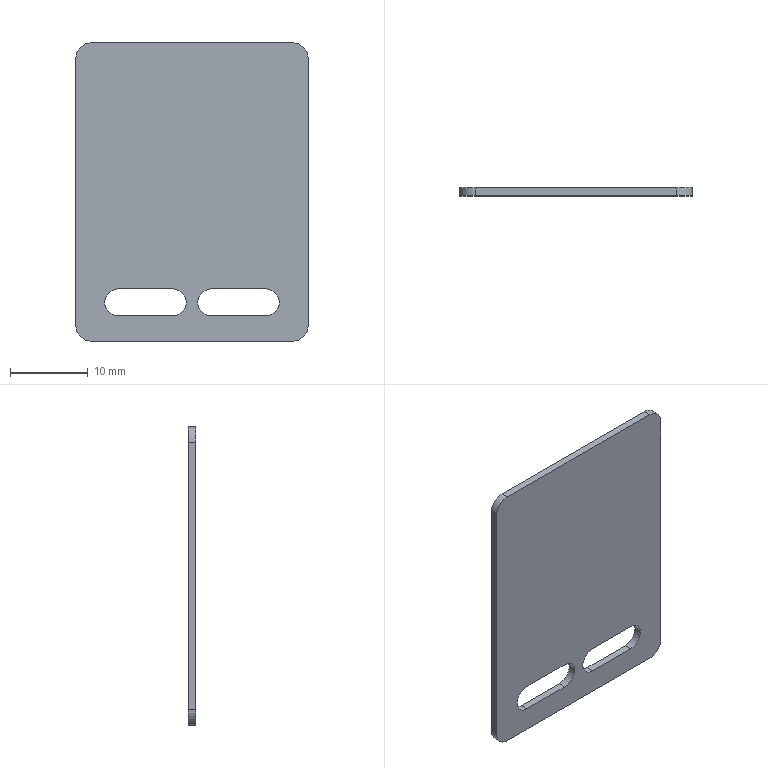Part | STEP file | 1 solid | 18 faces | box 30 x 1 x 38.5 mm | volume 1083 mm3 | plane 10 | cylinder 8 | commonest cylinder face diameters 3.5 x4 4 x4
STEP:
#1=CARTESIAN_POINT('',(0.,0.,0.));
#2=DIRECTION('',(0.,0.,1.));
#3=DIRECTION('',(1.,0.,0.));
#4=AXIS2_PLACEMENT_3D('',#1,#2,#3);
#5=CARTESIAN_POINT('',(-15.,-1.,2.));
#6=VERTEX_POINT('',#5);
#7=CARTESIAN_POINT('',(-13.,-1.,0.));
#8=VERTEX_POINT('',#7);
#9=CARTESIAN_POINT('',(-13.,-1.,2.));
#10=DIRECTION('',(0.,-1.,0.));
#11=DIRECTION('',(-1.,0.,0.));
#12=AXIS2_PLACEMENT_3D('',#9,#10,#11);
#13=CIRCLE('',#12,2.);
#14=CARTESIAN_POINT('',(-13.,0.,2.));
#15=DIRECTION('',(0.,1.,0.));
#16=DIRECTION('',(0.,0.,1.));
#17=AXIS2_PLACEMENT_3D('',#14,#15,#16);
#18=CYLINDRICAL_SURFACE('',#17,2.);
#19=CARTESIAN_POINT('',(4.712,-1.));
#20=DIRECTION('',(-1.,0.));
#21=VECTOR('',#20,1.);
#22=LINE('',#19,#21);
#23=(GEOMETRIC_REPRESENTATION_CONTEXT(2)PARAMETRIC_REPRESENTATION_CONTEXT()REPRESENTATION_CONTEXT('',''));
#24=DEFINITIONAL_REPRESENTATION('',(#22),#23);
#25=PCURVE('',#18,#24);
#26=CARTESIAN_POINT('',(-15.,-1.,38.5));
#27=DIRECTION('',(0.,1.,0.));
#28=DIRECTION('',(-1.,0.,0.));
#29=AXIS2_PLACEMENT_3D('',#26,#27,#28);
#30=PLANE('',#29);
#31=CARTESIAN_POINT('',(0.,-36.5));
#32=CARTESIAN_POINT('',(0.,-39.964));
#33=CARTESIAN_POINT('',(-3.,-38.232));
#34=CARTESIAN_POINT('',(-6.,-36.5));
#35=CARTESIAN_POINT('',(-3.,-34.768));
#36=CARTESIAN_POINT('',(0.,-33.036));
#37=CARTESIAN_POINT('',(0.,-36.5));
#38=(BOUNDED_CURVE()B_SPLINE_CURVE(2,(#31,#32,#33,#34,#35,#36,#37),.UNSPECIFIED.,.T.,.F.)B_SPLINE_CURVE_WITH_KNOTS((1,2,2,2,2,1),(-2.094,0.,2.094,4.189,6.283,8.378),.UNSPECIFIED.)CURVE()GEOMETRIC_REPRESENTATION_ITEM()RATIONAL_B_SPLINE_CURVE((1.,0.5,1.,0.5,1.,0.5,1.))REPRESENTATION_ITEM(''));
#39=(GEOMETRIC_REPRESENTATION_CONTEXT(2)PARAMETRIC_REPRESENTATION_CONTEXT()REPRESENTATION_CONTEXT('',''));
#40=DEFINITIONAL_REPRESENTATION('',(#38),#39);
#41=PCURVE('',#30,#40);
#42=SURFACE_CURVE('',#13,(#25,#41),.PCURVE_S1.);
#43=EDGE_CURVE('',#6,#8,#42,.T.);
#44=ORIENTED_EDGE('',*,*,#43,.F.);
#45=CARTESIAN_POINT('',(-15.,0.,2.));
#46=VERTEX_POINT('',#45);
#47=CARTESIAN_POINT('',(-15.,-1.,2.));
#48=DIRECTION('',(0.,-1.,0.));
#49=VECTOR('',#48,1.);
#50=LINE('',#47,#49);
#51=CARTESIAN_POINT('',(4.712,-1.));
#52=DIRECTION('',(0.,-1.));
#53=VECTOR('',#52,1.);
#54=LINE('',#51,#53);
#55=(GEOMETRIC_REPRESENTATION_CONTEXT(2)PARAMETRIC_REPRESENTATION_CONTEXT()REPRESENTATION_CONTEXT('',''));
#56=DEFINITIONAL_REPRESENTATION('',(#54),#55);
#57=PCURVE('',#18,#56);
#58=CARTESIAN_POINT('',(-15.,-1.,38.5));
#59=DIRECTION('',(-1.,0.,0.));
#60=DIRECTION('',(0.,0.,1.));
#61=AXIS2_PLACEMENT_3D('',#58,#59,#60);
#62=PLANE('',#61);
#63=CARTESIAN_POINT('',(-36.5,0.));
#64=DIRECTION('',(0.,-1.));
#65=VECTOR('',#64,1.);
#66=LINE('',#63,#65);
#67=(GEOMETRIC_REPRESENTATION_CONTEXT(2)PARAMETRIC_REPRESENTATION_CONTEXT()REPRESENTATION_CONTEXT('',''));
#68=DEFINITIONAL_REPRESENTATION('',(#66),#67);
#69=PCURVE('',#62,#68);
#70=SURFACE_CURVE('',#50,(#57,#69),.PCURVE_S1.);
#71=EDGE_CURVE('',#46,#6,#70,.T.);
#72=ORIENTED_EDGE('',*,*,#71,.F.);
#73=CARTESIAN_POINT('',(-13.,0.,0.));
#74=VERTEX_POINT('',#73);
#75=CARTESIAN_POINT('',(-13.,0.,2.));
#76=DIRECTION('',(0.,1.,0.));
#77=DIRECTION('',(-1.,0.,0.));
#78=AXIS2_PLACEMENT_3D('',#75,#76,#77);
#79=CIRCLE('',#78,2.);
#80=CARTESIAN_POINT('',(-1.571,0.));
#81=DIRECTION('',(1.,0.));
#82=VECTOR('',#81,1.);
#83=LINE('',#80,#82);
#84=(GEOMETRIC_REPRESENTATION_CONTEXT(2)PARAMETRIC_REPRESENTATION_CONTEXT()REPRESENTATION_CONTEXT('',''));
#85=DEFINITIONAL_REPRESENTATION('',(#83),#84);
#86=PCURVE('',#18,#85);
#87=CARTESIAN_POINT('',(-15.,0.,38.5));
#88=DIRECTION('',(0.,1.,0.));
#89=DIRECTION('',(-1.,0.,0.));
#90=AXIS2_PLACEMENT_3D('',#87,#88,#89);
#91=PLANE('',#90);
#92=CARTESIAN_POINT('',(-2.,-36.5));
#93=DIRECTION('',(1.,0.));
#94=AXIS2_PLACEMENT_2D('',#92,#93);
#95=CIRCLE('',#94,2.);
#96=(GEOMETRIC_REPRESENTATION_CONTEXT(2)PARAMETRIC_REPRESENTATION_CONTEXT()REPRESENTATION_CONTEXT('',''));
#97=DEFINITIONAL_REPRESENTATION('',(#95),#96);
#98=PCURVE('',#91,#97);
#99=SURFACE_CURVE('',#79,(#86,#98),.PCURVE_S1.);
#100=EDGE_CURVE('',#74,#46,#99,.T.);
#101=ORIENTED_EDGE('',*,*,#100,.F.);
#102=CARTESIAN_POINT('',(-13.,0.,0.));
#103=DIRECTION('',(0.,1.,0.));
#104=VECTOR('',#103,1.);
#105=LINE('',#102,#104);
#106=CARTESIAN_POINT('',(3.142,0.));
#107=DIRECTION('',(0.,1.));
#108=VECTOR('',#107,1.);
#109=LINE('',#106,#108);
#110=(GEOMETRIC_REPRESENTATION_CONTEXT(2)PARAMETRIC_REPRESENTATION_CONTEXT()REPRESENTATION_CONTEXT('',''));
#111=DEFINITIONAL_REPRESENTATION('',(#109),#110);
#112=PCURVE('',#18,#111);
#113=CARTESIAN_POINT('',(0.,0.,0.));
#114=DIRECTION('',(0.,0.,-1.));
#115=DIRECTION('',(-1.,0.,0.));
#116=AXIS2_PLACEMENT_3D('',#113,#114,#115);
#117=PLANE('',#116);
#118=CARTESIAN_POINT('',(13.,0.));
#119=DIRECTION('',(0.,1.));
#120=VECTOR('',#119,1.);
#121=LINE('',#118,#120);
#122=(GEOMETRIC_REPRESENTATION_CONTEXT(2)PARAMETRIC_REPRESENTATION_CONTEXT()REPRESENTATION_CONTEXT('',''));
#123=DEFINITIONAL_REPRESENTATION('',(#121),#122);
#124=PCURVE('',#117,#123);
#125=SURFACE_CURVE('',#105,(#112,#124),.PCURVE_S1.);
#126=EDGE_CURVE('',#8,#74,#125,.T.);
#127=ORIENTED_EDGE('',*,*,#126,.F.);
#128=EDGE_LOOP('',(#44,#72,#101,#127));
#129=FACE_BOUND('',#128,.T.);
#130=ADVANCED_FACE('',(#129),#18,.T.);
#131=CARTESIAN_POINT('',(15.,0.,2.));
#132=VERTEX_POINT('',#131);
#133=CARTESIAN_POINT('',(13.,0.,0.));
#134=VERTEX_POINT('',#133);
#135=CARTESIAN_POINT('',(13.,0.,2.));
#136=DIRECTION('',(0.,1.,0.));
#137=DIRECTION('',(-1.,0.,0.));
#138=AXIS2_PLACEMENT_3D('',#135,#136,#137);
#139=CIRCLE('',#138,2.);
#140=CARTESIAN_POINT('',(13.,0.,2.));
#141=DIRECTION('',(0.,-1.,0.));
#142=DIRECTION('',(0.,0.,-1.));
#143=AXIS2_PLACEMENT_3D('',#140,#141,#142);
#144=CYLINDRICAL_SURFACE('',#143,2.);
#145=CARTESIAN_POINT('',(4.712,0.));
#146=DIRECTION('',(-1.,0.));
#147=VECTOR('',#146,1.);
#148=LINE('',#145,#147);
#149=(GEOMETRIC_REPRESENTATION_CONTEXT(2)PARAMETRIC_REPRESENTATION_CONTEXT()REPRESENTATION_CONTEXT('',''));
#150=DEFINITIONAL_REPRESENTATION('',(#148),#149);
#151=PCURVE('',#144,#150);
#152=CARTESIAN_POINT('',(-28.,-36.5));
#153=DIRECTION('',(1.,0.));
#154=AXIS2_PLACEMENT_2D('',#152,#153);
#155=CIRCLE('',#154,2.);
#156=(GEOMETRIC_REPRESENTATION_CONTEXT(2)PARAMETRIC_REPRESENTATION_CONTEXT()REPRESENTATION_CONTEXT('',''));
#157=DEFINITIONAL_REPRESENTATION('',(#155),#156);
#158=PCURVE('',#91,#157);
#159=SURFACE_CURVE('',#139,(#151,#158),.PCURVE_S1.);
#160=EDGE_CURVE('',#132,#134,#159,.T.);
#161=ORIENTED_EDGE('',*,*,#160,.F.);
#162=CARTESIAN_POINT('',(15.,-1.,2.));
#163=VERTEX_POINT('',#162);
#164=CARTESIAN_POINT('',(15.,0.,2.));
#165=DIRECTION('',(0.,1.,0.));
#166=VECTOR('',#165,1.);
#167=LINE('',#164,#166);
#168=CARTESIAN_POINT('',(1.571,0.));
#169=DIRECTION('',(0.,-1.));
#170=VECTOR('',#169,1.);
#171=LINE('',#168,#170);
#172=(GEOMETRIC_REPRESENTATION_CONTEXT(2)PARAMETRIC_REPRESENTATION_CONTEXT()REPRESENTATION_CONTEXT('',''));
#173=DEFINITIONAL_REPRESENTATION('',(#171),#172);
#174=PCURVE('',#144,#173);
#175=CARTESIAN_POINT('',(15.,0.,38.5));
#176=DIRECTION('',(1.,0.,0.));
#177=DIRECTION('',(0.,0.,-1.));
#178=AXIS2_PLACEMENT_3D('',#175,#176,#177);
#179=PLANE('',#178);
#180=CARTESIAN_POINT('',(36.5,0.));
#181=DIRECTION('',(0.,1.));
#182=VECTOR('',#181,1.);
#183=LINE('',#180,#182);
#184=(GEOMETRIC_REPRESENTATION_CONTEXT(2)PARAMETRIC_REPRESENTATION_CONTEXT()REPRESENTATION_CONTEXT('',''));
#185=DEFINITIONAL_REPRESENTATION('',(#183),#184);
#186=PCURVE('',#179,#185);
#187=SURFACE_CURVE('',#167,(#174,#186),.PCURVE_S1.);
#188=EDGE_CURVE('',#163,#132,#187,.T.);
#189=ORIENTED_EDGE('',*,*,#188,.F.);
#190=CARTESIAN_POINT('',(13.,-1.,0.));
#191=VERTEX_POINT('',#190);
#192=CARTESIAN_POINT('',(13.,-1.,2.));
#193=DIRECTION('',(0.,-1.,0.));
#194=DIRECTION('',(-1.,0.,0.));
#195=AXIS2_PLACEMENT_3D('',#192,#193,#194);
#196=CIRCLE('',#195,2.);
#197=CARTESIAN_POINT('',(-1.571,1.));
#198=DIRECTION('',(1.,0.));
#199=VECTOR('',#198,1.);
#200=LINE('',#197,#199);
#201=(GEOMETRIC_REPRESENTATION_CONTEXT(2)PARAMETRIC_REPRESENTATION_CONTEXT()REPRESENTATION_CONTEXT('',''));
#202=DEFINITIONAL_REPRESENTATION('',(#200),#201);
#203=PCURVE('',#144,#202);
#204=CARTESIAN_POINT('',(-26.,-36.5));
#205=CARTESIAN_POINT('',(-26.,-39.964));
#206=CARTESIAN_POINT('',(-29.,-38.232));
#207=CARTESIAN_POINT('',(-32.,-36.5));
#208=CARTESIAN_POINT('',(-29.,-34.768));
#209=CARTESIAN_POINT('',(-26.,-33.036));
#210=CARTESIAN_POINT('',(-26.,-36.5));
#211=(BOUNDED_CURVE()B_SPLINE_CURVE(2,(#204,#205,#206,#207,#208,#209,#210),.UNSPECIFIED.,.T.,.F.)B_SPLINE_CURVE_WITH_KNOTS((1,2,2,2,2,1),(-2.094,0.,2.094,4.189,6.283,8.378),.UNSPECIFIED.)CURVE()GEOMETRIC_REPRESENTATION_ITEM()RATIONAL_B_SPLINE_CURVE((1.,0.5,1.,0.5,1.,0.5,1.))REPRESENTATION_ITEM(''));
#212=(GEOMETRIC_REPRESENTATION_CONTEXT(2)PARAMETRIC_REPRESENTATION_CONTEXT()REPRESENTATION_CONTEXT('',''));
#213=DEFINITIONAL_REPRESENTATION('',(#211),#212);
#214=PCURVE('',#30,#213);
#215=SURFACE_CURVE('',#196,(#203,#214),.PCURVE_S1.);
#216=EDGE_CURVE('',#191,#163,#215,.T.);
#217=ORIENTED_EDGE('',*,*,#216,.F.);
#218=CARTESIAN_POINT('',(13.,0.,0.));
#219=DIRECTION('',(0.,-1.,0.));
#220=VECTOR('',#219,1.);
#221=LINE('',#218,#220);
#222=CARTESIAN_POINT('',(0.,0.));
#223=DIRECTION('',(0.,1.));
#224=VECTOR('',#223,1.);
#225=LINE('',#222,#224);
#226=(GEOMETRIC_REPRESENTATION_CONTEXT(2)PARAMETRIC_REPRESENTATION_CONTEXT()REPRESENTATION_CONTEXT('',''));
#227=DEFINITIONAL_REPRESENTATION('',(#225),#226);
#228=PCURVE('',#144,#227);
#229=CARTESIAN_POINT('',(-13.,0.));
#230=DIRECTION('',(0.,-1.));
#231=VECTOR('',#230,1.);
#232=LINE('',#229,#231);
#233=(GEOMETRIC_REPRESENTATION_CONTEXT(2)PARAMETRIC_REPRESENTATION_CONTEXT()REPRESENTATION_CONTEXT('',''));
#234=DEFINITIONAL_REPRESENTATION('',(#232),#233);
#235=PCURVE('',#117,#234);
#236=SURFACE_CURVE('',#221,(#228,#235),.PCURVE_S1.);
#237=EDGE_CURVE('',#134,#191,#236,.T.);
#238=ORIENTED_EDGE('',*,*,#237,.F.);
#239=EDGE_LOOP('',(#161,#189,#217,#238));
#240=FACE_BOUND('',#239,.T.);
#241=ADVANCED_FACE('',(#240),#144,.T.);
#242=CARTESIAN_POINT('',(-13.,-1.,38.5));
#243=VERTEX_POINT('',#242);
#244=CARTESIAN_POINT('',(-15.,-1.,36.5));
#245=VERTEX_POINT('',#244);
#246=CARTESIAN_POINT('',(-13.,-1.,36.5));
#247=DIRECTION('',(0.,-1.,0.));
#248=DIRECTION('',(-1.,0.,0.));
#249=AXIS2_PLACEMENT_3D('',#246,#247,#248);
#250=CIRCLE('',#249,2.);
#251=CARTESIAN_POINT('',(-13.,-1.,36.5));
#252=DIRECTION('',(0.,-1.,0.));
#253=DIRECTION('',(0.,0.,-1.));
#254=AXIS2_PLACEMENT_3D('',#251,#252,#253);
#255=CYLINDRICAL_SURFACE('',#254,2.);
#256=CARTESIAN_POINT('',(-1.571,0.));
#257=DIRECTION('',(1.,0.));
#258=VECTOR('',#257,1.);
#259=LINE('',#256,#258);
#260=(GEOMETRIC_REPRESENTATION_CONTEXT(2)PARAMETRIC_REPRESENTATION_CONTEXT()REPRESENTATION_CONTEXT('',''));
#261=DEFINITIONAL_REPRESENTATION('',(#259),#260);
#262=PCURVE('',#255,#261);
#263=CARTESIAN_POINT('',(0.,-2.));
#264=CARTESIAN_POINT('',(0.,-5.464));
#265=CARTESIAN_POINT('',(-3.,-3.732));
#266=CARTESIAN_POINT('',(-6.,-2.));
#267=CARTESIAN_POINT('',(-3.,-0.2679));
#268=CARTESIAN_POINT('',(0.,1.464));
#269=CARTESIAN_POINT('',(0.,-2.));
#270=(BOUNDED_CURVE()B_SPLINE_CURVE(2,(#263,#264,#265,#266,#267,#268,#269),.UNSPECIFIED.,.T.,.F.)B_SPLINE_CURVE_WITH_KNOTS((1,2,2,2,2,1),(-2.094,0.,2.094,4.189,6.283,8.378),.UNSPECIFIED.)CURVE()GEOMETRIC_REPRESENTATION_ITEM()RATIONAL_B_SPLINE_CURVE((1.,0.5,1.,0.5,1.,0.5,1.))REPRESENTATION_ITEM(''));
#271=(GEOMETRIC_REPRESENTATION_CONTEXT(2)PARAMETRIC_REPRESENTATION_CONTEXT()REPRESENTATION_CONTEXT('',''));
#272=DEFINITIONAL_REPRESENTATION('',(#270),#271);
#273=PCURVE('',#30,#272);
#274=SURFACE_CURVE('',#250,(#262,#273),.PCURVE_S1.);
#275=EDGE_CURVE('',#243,#245,#274,.T.);
#276=ORIENTED_EDGE('',*,*,#275,.F.);
#277=CARTESIAN_POINT('',(-13.,0.,38.5));
#278=VERTEX_POINT('',#277);
#279=CARTESIAN_POINT('',(-13.,-1.,38.5));
#280=DIRECTION('',(0.,-1.,0.));
#281=VECTOR('',#280,1.);
#282=LINE('',#279,#281);
#283=CARTESIAN_POINT('',(3.142,0.));
#284=DIRECTION('',(0.,1.));
#285=VECTOR('',#284,1.);
#286=LINE('',#283,#285);
#287=(GEOMETRIC_REPRESENTATION_CONTEXT(2)PARAMETRIC_REPRESENTATION_CONTEXT()REPRESENTATION_CONTEXT('',''));
#288=DEFINITIONAL_REPRESENTATION('',(#286),#287);
#289=PCURVE('',#255,#288);
#290=CARTESIAN_POINT('',(0.,0.,38.5));
#291=DIRECTION('',(0.,0.,-1.));
#292=DIRECTION('',(-1.,0.,0.));
#293=AXIS2_PLACEMENT_3D('',#290,#291,#292);
#294=PLANE('',#293);
#295=CARTESIAN_POINT('',(13.,-1.));
#296=DIRECTION('',(0.,-1.));
#297=VECTOR('',#296,1.);
#298=LINE('',#295,#297);
#299=(GEOMETRIC_REPRESENTATION_CONTEXT(2)PARAMETRIC_REPRESENTATION_CONTEXT()REPRESENTATION_CONTEXT('',''));
#300=DEFINITIONAL_REPRESENTATION('',(#298),#299);
#301=PCURVE('',#294,#300);
#302=SURFACE_CURVE('',#282,(#289,#301),.PCURVE_S1.);
#303=EDGE_CURVE('',#278,#243,#302,.T.);
#304=ORIENTED_EDGE('',*,*,#303,.F.);
#305=CARTESIAN_POINT('',(-15.,0.,36.5));
#306=VERTEX_POINT('',#305);
#307=CARTESIAN_POINT('',(-13.,0.,36.5));
#308=DIRECTION('',(0.,1.,0.));
#309=DIRECTION('',(-1.,0.,0.));
#310=AXIS2_PLACEMENT_3D('',#307,#308,#309);
#311=CIRCLE('',#310,2.);
#312=CARTESIAN_POINT('',(4.712,-1.));
#313=DIRECTION('',(-1.,0.));
#314=VECTOR('',#313,1.);
#315=LINE('',#312,#314);
#316=(GEOMETRIC_REPRESENTATION_CONTEXT(2)PARAMETRIC_REPRESENTATION_CONTEXT()REPRESENTATION_CONTEXT('',''));
#317=DEFINITIONAL_REPRESENTATION('',(#315),#316);
#318=PCURVE('',#255,#317);
#319=CARTESIAN_POINT('',(-2.,-2.));
#320=DIRECTION('',(1.,0.));
#321=AXIS2_PLACEMENT_2D('',#319,#320);
#322=CIRCLE('',#321,2.);
#323=(GEOMETRIC_REPRESENTATION_CONTEXT(2)PARAMETRIC_REPRESENTATION_CONTEXT()REPRESENTATION_CONTEXT('',''));
#324=DEFINITIONAL_REPRESENTATION('',(#322),#323);
#325=PCURVE('',#91,#324);
#326=SURFACE_CURVE('',#311,(#318,#325),.PCURVE_S1.);
#327=EDGE_CURVE('',#306,#278,#326,.T.);
#328=ORIENTED_EDGE('',*,*,#327,.F.);
#329=CARTESIAN_POINT('',(-15.,0.,36.5));
#330=DIRECTION('',(0.,1.,0.));
#331=VECTOR('',#330,1.);
#332=LINE('',#329,#331);
#333=CARTESIAN_POINT('',(4.712,-1.));
#334=DIRECTION('',(0.,-1.));
#335=VECTOR('',#334,1.);
#336=LINE('',#333,#335);
#337=(GEOMETRIC_REPRESENTATION_CONTEXT(2)PARAMETRIC_REPRESENTATION_CONTEXT()REPRESENTATION_CONTEXT('',''));
#338=DEFINITIONAL_REPRESENTATION('',(#336),#337);
#339=PCURVE('',#255,#338);
#340=CARTESIAN_POINT('',(-2.,1.));
#341=DIRECTION('',(0.,1.));
#342=VECTOR('',#341,1.);
#343=LINE('',#340,#342);
#344=(GEOMETRIC_REPRESENTATION_CONTEXT(2)PARAMETRIC_REPRESENTATION_CONTEXT()REPRESENTATION_CONTEXT('',''));
#345=DEFINITIONAL_REPRESENTATION('',(#343),#344);
#346=PCURVE('',#62,#345);
#347=SURFACE_CURVE('',#332,(#339,#346),.PCURVE_S1.);
#348=EDGE_CURVE('',#245,#306,#347,.T.);
#349=ORIENTED_EDGE('',*,*,#348,.F.);
#350=EDGE_LOOP('',(#276,#304,#328,#349));
#351=FACE_BOUND('',#350,.T.);
#352=ADVANCED_FACE('',(#351),#255,.T.);
#353=CARTESIAN_POINT('',(13.,0.,38.5));
#354=VERTEX_POINT('',#353);
#355=CARTESIAN_POINT('',(15.,0.,36.5));
#356=VERTEX_POINT('',#355);
#357=CARTESIAN_POINT('',(13.,0.,36.5));
#358=DIRECTION('',(0.,1.,0.));
#359=DIRECTION('',(-1.,0.,0.));
#360=AXIS2_PLACEMENT_3D('',#357,#358,#359);
#361=CIRCLE('',#360,2.);
#362=CARTESIAN_POINT('',(13.,0.,36.5));
#363=DIRECTION('',(0.,1.,0.));
#364=DIRECTION('',(0.,0.,1.));
#365=AXIS2_PLACEMENT_3D('',#362,#363,#364);
#366=CYLINDRICAL_SURFACE('',#365,2.);
#367=CARTESIAN_POINT('',(-1.571,0.));
#368=DIRECTION('',(1.,0.));
#369=VECTOR('',#368,1.);
#370=LINE('',#367,#369);
#371=(GEOMETRIC_REPRESENTATION_CONTEXT(2)PARAMETRIC_REPRESENTATION_CONTEXT()REPRESENTATION_CONTEXT('',''));
#372=DEFINITIONAL_REPRESENTATION('',(#370),#371);
#373=PCURVE('',#366,#372);
#374=CARTESIAN_POINT('',(-28.,-2.));
#375=DIRECTION('',(1.,0.));
#376=AXIS2_PLACEMENT_2D('',#374,#375);
#377=CIRCLE('',#376,2.);
#378=(GEOMETRIC_REPRESENTATION_CONTEXT(2)PARAMETRIC_REPRESENTATION_CONTEXT()REPRESENTATION_CONTEXT('',''));
#379=DEFINITIONAL_REPRESENTATION('',(#377),#378);
#380=PCURVE('',#91,#379);
#381=SURFACE_CURVE('',#361,(#373,#380),.PCURVE_S1.);
#382=EDGE_CURVE('',#354,#356,#381,.T.);
#383=ORIENTED_EDGE('',*,*,#382,.F.);
#384=CARTESIAN_POINT('',(13.,-1.,38.5));
#385=VERTEX_POINT('',#384);
#386=CARTESIAN_POINT('',(13.,0.,38.5));
#387=DIRECTION('',(0.,1.,0.));
#388=VECTOR('',#387,1.);
#389=LINE('',#386,#388);
#390=CARTESIAN_POINT('',(0.,0.));
#391=DIRECTION('',(0.,1.));
#392=VECTOR('',#391,1.);
#393=LINE('',#390,#392);
#394=(GEOMETRIC_REPRESENTATION_CONTEXT(2)PARAMETRIC_REPRESENTATION_CONTEXT()REPRESENTATION_CONTEXT('',''));
#395=DEFINITIONAL_REPRESENTATION('',(#393),#394);
#396=PCURVE('',#366,#395);
#397=CARTESIAN_POINT('',(-13.,0.));
#398=DIRECTION('',(0.,1.));
#399=VECTOR('',#398,1.);
#400=LINE('',#397,#399);
#401=(GEOMETRIC_REPRESENTATION_CONTEXT(2)PARAMETRIC_REPRESENTATION_CONTEXT()REPRESENTATION_CONTEXT('',''));
#402=DEFINITIONAL_REPRESENTATION('',(#400),#401);
#403=PCURVE('',#294,#402);
#404=SURFACE_CURVE('',#389,(#396,#403),.PCURVE_S1.);
#405=EDGE_CURVE('',#385,#354,#404,.T.);
#406=ORIENTED_EDGE('',*,*,#405,.F.);
#407=CARTESIAN_POINT('',(15.,-1.,36.5));
#408=VERTEX_POINT('',#407);
#409=CARTESIAN_POINT('',(13.,-1.,36.5));
#410=DIRECTION('',(0.,-1.,0.));
#411=DIRECTION('',(-1.,0.,0.));
#412=AXIS2_PLACEMENT_3D('',#409,#410,#411);
#413=CIRCLE('',#412,2.);
#414=CARTESIAN_POINT('',(4.712,-1.));
#415=DIRECTION('',(-1.,0.));
#416=VECTOR('',#415,1.);
#417=LINE('',#414,#416);
#418=(GEOMETRIC_REPRESENTATION_CONTEXT(2)PARAMETRIC_REPRESENTATION_CONTEXT()REPRESENTATION_CONTEXT('',''));
#419=DEFINITIONAL_REPRESENTATION('',(#417),#418);
#420=PCURVE('',#366,#419);
#421=CARTESIAN_POINT('',(-26.,-2.));
#422=CARTESIAN_POINT('',(-26.,-5.464));
#423=CARTESIAN_POINT('',(-29.,-3.732));
#424=CARTESIAN_POINT('',(-32.,-2.));
#425=CARTESIAN_POINT('',(-29.,-0.2679));
#426=CARTESIAN_POINT('',(-26.,1.464));
#427=CARTESIAN_POINT('',(-26.,-2.));
#428=(BOUNDED_CURVE()B_SPLINE_CURVE(2,(#421,#422,#423,#424,#425,#426,#427),.UNSPECIFIED.,.T.,.F.)B_SPLINE_CURVE_WITH_KNOTS((1,2,2,2,2,1),(-2.094,0.,2.094,4.189,6.283,8.378),.UNSPECIFIED.)CURVE()GEOMETRIC_REPRESENTATION_ITEM()RATIONAL_B_SPLINE_CURVE((1.,0.5,1.,0.5,1.,0.5,1.))REPRESENTATION_ITEM(''));
#429=(GEOMETRIC_REPRESENTATION_CONTEXT(2)PARAMETRIC_REPRESENTATION_CONTEXT()REPRESENTATION_CONTEXT('',''));
#430=DEFINITIONAL_REPRESENTATION('',(#428),#429);
#431=PCURVE('',#30,#430);
#432=SURFACE_CURVE('',#413,(#420,#431),.PCURVE_S1.);
#433=EDGE_CURVE('',#408,#385,#432,.T.);
#434=ORIENTED_EDGE('',*,*,#433,.F.);
#435=CARTESIAN_POINT('',(15.,-1.,36.5));
#436=DIRECTION('',(0.,-1.,0.));
#437=VECTOR('',#436,1.);
#438=LINE('',#435,#437);
#439=CARTESIAN_POINT('',(1.571,-1.));
#440=DIRECTION('',(0.,-1.));
#441=VECTOR('',#440,1.);
#442=LINE('',#439,#441);
#443=(GEOMETRIC_REPRESENTATION_CONTEXT(2)PARAMETRIC_REPRESENTATION_CONTEXT()REPRESENTATION_CONTEXT('',''));
#444=DEFINITIONAL_REPRESENTATION('',(#442),#443);
#445=PCURVE('',#366,#444);
#446=CARTESIAN_POINT('',(2.,-1.));
#447=DIRECTION('',(0.,-1.));
#448=VECTOR('',#447,1.);
#449=LINE('',#446,#448);
#450=(GEOMETRIC_REPRESENTATION_CONTEXT(2)PARAMETRIC_REPRESENTATION_CONTEXT()REPRESENTATION_CONTEXT('',''));
#451=DEFINITIONAL_REPRESENTATION('',(#449),#450);
#452=PCURVE('',#179,#451);
#453=SURFACE_CURVE('',#438,(#445,#452),.PCURVE_S1.);
#454=EDGE_CURVE('',#356,#408,#453,.T.);
#455=ORIENTED_EDGE('',*,*,#454,.F.);
#456=EDGE_LOOP('',(#383,#406,#434,#455));
#457=FACE_BOUND('',#456,.T.);
#458=ADVANCED_FACE('',(#457),#366,.T.);
#459=CARTESIAN_POINT('',(2.5,-1.,6.75));
#460=VERTEX_POINT('',#459);
#461=CARTESIAN_POINT('',(2.5,0.,6.75));
#462=VERTEX_POINT('',#461);
#463=CARTESIAN_POINT('',(2.5,-10.,6.75));
#464=DIRECTION('',(0.,1.,0.));
#465=VECTOR('',#464,1.);
#466=LINE('',#463,#465);
#467=CARTESIAN_POINT('',(2.5,-10.,6.75));
#468=DIRECTION('',(0.,0.,1.));
#469=DIRECTION('',(1.,0.,0.));
#470=AXIS2_PLACEMENT_3D('',#467,#468,#469);
#471=PLANE('',#470);
#472=CARTESIAN_POINT('',(0.,0.));
#473=DIRECTION('',(0.,1.));
#474=VECTOR('',#473,1.);
#475=LINE('',#472,#474);
#476=(GEOMETRIC_REPRESENTATION_CONTEXT(2)PARAMETRIC_REPRESENTATION_CONTEXT()REPRESENTATION_CONTEXT('',''));
#477=DEFINITIONAL_REPRESENTATION('',(#475),#476);
#478=PCURVE('',#471,#477);
#479=CARTESIAN_POINT('',(2.5,-10.,5.));
#480=DIRECTION('',(0.,1.,0.));
#481=DIRECTION('',(0.,0.,1.));
#482=AXIS2_PLACEMENT_3D('',#479,#480,#481);
#483=CYLINDRICAL_SURFACE('',#482,1.75);
#484=CARTESIAN_POINT('',(6.283,0.));
#485=DIRECTION('',(0.,1.));
#486=VECTOR('',#485,1.);
#487=LINE('',#484,#486);
#488=(GEOMETRIC_REPRESENTATION_CONTEXT(2)PARAMETRIC_REPRESENTATION_CONTEXT()REPRESENTATION_CONTEXT('',''));
#489=DEFINITIONAL_REPRESENTATION('',(#487),#488);
#490=PCURVE('',#483,#489);
#491=SURFACE_CURVE('',#466,(#478,#490),.PCURVE_S1.);
#492=EDGE_CURVE('',#460,#462,#491,.T.);
#493=ORIENTED_EDGE('',*,*,#492,.T.);
#494=CARTESIAN_POINT('',(9.5,0.,6.75));
#495=VERTEX_POINT('',#494);
#496=CARTESIAN_POINT('',(2.5,0.,6.75));
#497=DIRECTION('',(1.,0.,0.));
#498=VECTOR('',#497,1.);
#499=LINE('',#496,#498);
#500=CARTESIAN_POINT('',(0.,10.));
#501=DIRECTION('',(1.,0.));
#502=VECTOR('',#501,1.);
#503=LINE('',#500,#502);
#504=(GEOMETRIC_REPRESENTATION_CONTEXT(2)PARAMETRIC_REPRESENTATION_CONTEXT()REPRESENTATION_CONTEXT('',''));
#505=DEFINITIONAL_REPRESENTATION('',(#503),#504);
#506=PCURVE('',#471,#505);
#507=CARTESIAN_POINT('',(-17.5,-31.75));
#508=DIRECTION('',(-1.,0.));
#509=VECTOR('',#508,1.);
#510=LINE('',#507,#509);
#511=(GEOMETRIC_REPRESENTATION_CONTEXT(2)PARAMETRIC_REPRESENTATION_CONTEXT()REPRESENTATION_CONTEXT('',''));
#512=DEFINITIONAL_REPRESENTATION('',(#510),#511);
#513=PCURVE('',#91,#512);
#514=SURFACE_CURVE('',#499,(#506,#513),.PCURVE_S1.);
#515=EDGE_CURVE('',#462,#495,#514,.T.);
#516=ORIENTED_EDGE('',*,*,#515,.T.);
#517=CARTESIAN_POINT('',(9.5,-1.,6.75));
#518=VERTEX_POINT('',#517);
#519=CARTESIAN_POINT('',(9.5,-10.,6.75));
#520=DIRECTION('',(0.,1.,0.));
#521=VECTOR('',#520,1.);
#522=LINE('',#519,#521);
#523=CARTESIAN_POINT('',(7.,0.));
#524=DIRECTION('',(0.,1.));
#525=VECTOR('',#524,1.);
#526=LINE('',#523,#525);
#527=(GEOMETRIC_REPRESENTATION_CONTEXT(2)PARAMETRIC_REPRESENTATION_CONTEXT()REPRESENTATION_CONTEXT('',''));
#528=DEFINITIONAL_REPRESENTATION('',(#526),#527);
#529=PCURVE('',#471,#528);
#530=CARTESIAN_POINT('',(9.5,-10.,5.));
#531=DIRECTION('',(0.,1.,0.));
#532=DIRECTION('',(0.,0.,1.));
#533=AXIS2_PLACEMENT_3D('',#530,#531,#532);
#534=CYLINDRICAL_SURFACE('',#533,1.75);
#535=CARTESIAN_POINT('',(0.,0.));
#536=DIRECTION('',(0.,1.));
#537=VECTOR('',#536,1.);
#538=LINE('',#535,#537);
#539=(GEOMETRIC_REPRESENTATION_CONTEXT(2)PARAMETRIC_REPRESENTATION_CONTEXT()REPRESENTATION_CONTEXT('',''));
#540=DEFINITIONAL_REPRESENTATION('',(#538),#539);
#541=PCURVE('',#534,#540);
#542=SURFACE_CURVE('',#522,(#529,#541),.PCURVE_S1.);
#543=EDGE_CURVE('',#518,#495,#542,.T.);
#544=ORIENTED_EDGE('',*,*,#543,.F.);
#545=CARTESIAN_POINT('',(-15.,-1.,6.75));
#546=DIRECTION('',(1.,0.,0.));
#547=VECTOR('',#546,1.);
#548=LINE('',#545,#547);
#549=CARTESIAN_POINT('',(-17.5,9.));
#550=DIRECTION('',(1.,0.));
#551=VECTOR('',#550,1.);
#552=LINE('',#549,#551);
#553=(GEOMETRIC_REPRESENTATION_CONTEXT(2)PARAMETRIC_REPRESENTATION_CONTEXT()REPRESENTATION_CONTEXT('',''));
#554=DEFINITIONAL_REPRESENTATION('',(#552),#553);
#555=PCURVE('',#471,#554);
#556=CARTESIAN_POINT('',(0.,-31.75));
#557=DIRECTION('',(-1.,0.));
#558=VECTOR('',#557,1.);
#559=LINE('',#556,#558);
#560=(GEOMETRIC_REPRESENTATION_CONTEXT(2)PARAMETRIC_REPRESENTATION_CONTEXT()REPRESENTATION_CONTEXT('',''));
#561=DEFINITIONAL_REPRESENTATION('',(#559),#560);
#562=PCURVE('',#30,#561);
#563=SURFACE_CURVE('',#548,(#555,#562),.PCURVE_S1.);
#564=EDGE_CURVE('',#460,#518,#563,.T.);
#565=ORIENTED_EDGE('',*,*,#564,.F.);
#566=EDGE_LOOP('',(#493,#516,#544,#565));
#567=FACE_BOUND('',#566,.T.);
#568=ADVANCED_FACE('',(#567),#471,.F.);
#569=CARTESIAN_POINT('',(9.5,-1.,3.25));
#570=VERTEX_POINT('',#569);
#571=CARTESIAN_POINT('',(9.5,-1.,5.));
#572=DIRECTION('',(0.,1.,0.));
#573=DIRECTION('',(-1.,0.,0.));
#574=AXIS2_PLACEMENT_3D('',#571,#572,#573);
#575=CIRCLE('',#574,1.75);
#576=CARTESIAN_POINT('',(-1.571,9.));
#577=DIRECTION('',(1.,0.));
#578=VECTOR('',#577,1.);
#579=LINE('',#576,#578);
#580=(GEOMETRIC_REPRESENTATION_CONTEXT(2)PARAMETRIC_REPRESENTATION_CONTEXT()REPRESENTATION_CONTEXT('',''));
#581=DEFINITIONAL_REPRESENTATION('',(#579),#580);
#582=PCURVE('',#534,#581);
#583=CARTESIAN_POINT('',(-24.5,-33.5));
#584=DIRECTION('',(1.,0.));
#585=AXIS2_PLACEMENT_2D('',#583,#584);
#586=CIRCLE('',#585,1.75);
#587=(GEOMETRIC_REPRESENTATION_CONTEXT(2)PARAMETRIC_REPRESENTATION_CONTEXT()REPRESENTATION_CONTEXT('',''));
#588=DEFINITIONAL_REPRESENTATION('',(#586),#587);
#589=PCURVE('',#30,#588);
#590=SURFACE_CURVE('',#575,(#582,#589),.PCURVE_S1.);
#591=EDGE_CURVE('',#518,#570,#590,.T.);
#592=ORIENTED_EDGE('',*,*,#591,.T.);
#593=CARTESIAN_POINT('',(9.5,0.,3.25));
#594=VERTEX_POINT('',#593);
#595=CARTESIAN_POINT('',(9.5,-10.,3.25));
#596=DIRECTION('',(0.,1.,0.));
#597=VECTOR('',#596,1.);
#598=LINE('',#595,#597);
#599=CARTESIAN_POINT('',(3.142,0.));
#600=DIRECTION('',(0.,1.));
#601=VECTOR('',#600,1.);
#602=LINE('',#599,#601);
#603=(GEOMETRIC_REPRESENTATION_CONTEXT(2)PARAMETRIC_REPRESENTATION_CONTEXT()REPRESENTATION_CONTEXT('',''));
#604=DEFINITIONAL_REPRESENTATION('',(#602),#603);
#605=PCURVE('',#534,#604);
#606=CARTESIAN_POINT('',(2.5,-10.,3.25));
#607=DIRECTION('',(0.,0.,-1.));
#608=DIRECTION('',(-1.,0.,0.));
#609=AXIS2_PLACEMENT_3D('',#606,#607,#608);
#610=PLANE('',#609);
#611=CARTESIAN_POINT('',(-7.,0.));
#612=DIRECTION('',(0.,1.));
#613=VECTOR('',#612,1.);
#614=LINE('',#611,#613);
#615=(GEOMETRIC_REPRESENTATION_CONTEXT(2)PARAMETRIC_REPRESENTATION_CONTEXT()REPRESENTATION_CONTEXT('',''));
#616=DEFINITIONAL_REPRESENTATION('',(#614),#615);
#617=PCURVE('',#610,#616);
#618=SURFACE_CURVE('',#598,(#605,#617),.PCURVE_S1.);
#619=EDGE_CURVE('',#570,#594,#618,.T.);
#620=ORIENTED_EDGE('',*,*,#619,.T.);
#621=CARTESIAN_POINT('',(9.5,0.,5.));
#622=DIRECTION('',(0.,1.,0.));
#623=DIRECTION('',(0.,0.,1.));
#624=AXIS2_PLACEMENT_3D('',#621,#622,#623);
#625=CIRCLE('',#624,1.75);
#626=CARTESIAN_POINT('',(0.,10.));
#627=DIRECTION('',(1.,0.));
#628=VECTOR('',#627,1.);
#629=LINE('',#626,#628);
#630=(GEOMETRIC_REPRESENTATION_CONTEXT(2)PARAMETRIC_REPRESENTATION_CONTEXT()REPRESENTATION_CONTEXT('',''));
#631=DEFINITIONAL_REPRESENTATION('',(#629),#630);
#632=PCURVE('',#534,#631);
#633=CARTESIAN_POINT('',(-24.5,-33.5));
#634=DIRECTION('',(0.,1.));
#635=AXIS2_PLACEMENT_2D('',#633,#634);
#636=CIRCLE('',#635,1.75);
#637=(GEOMETRIC_REPRESENTATION_CONTEXT(2)PARAMETRIC_REPRESENTATION_CONTEXT()REPRESENTATION_CONTEXT('',''));
#638=DEFINITIONAL_REPRESENTATION('',(#636),#637);
#639=PCURVE('',#91,#638);
#640=SURFACE_CURVE('',#625,(#632,#639),.PCURVE_S1.);
#641=EDGE_CURVE('',#495,#594,#640,.T.);
#642=ORIENTED_EDGE('',*,*,#641,.F.);
#643=ORIENTED_EDGE('',*,*,#543,.F.);
#644=EDGE_LOOP('',(#592,#620,#642,#643));
#645=FACE_BOUND('',#644,.F.);
#646=ADVANCED_FACE('',(#645),#534,.F.);
#647=ORIENTED_EDGE('',*,*,#619,.T.);
#648=CARTESIAN_POINT('',(2.5,0.,3.25));
#649=VERTEX_POINT('',#648);
#650=CARTESIAN_POINT('',(2.5,0.,3.25));
#651=DIRECTION('',(-1.,0.,0.));
#652=VECTOR('',#651,1.);
#653=LINE('',#650,#652);
#654=CARTESIAN_POINT('',(0.,10.));
#655=DIRECTION('',(1.,0.));
#656=VECTOR('',#655,1.);
#657=LINE('',#654,#656);
#658=(GEOMETRIC_REPRESENTATION_CONTEXT(2)PARAMETRIC_REPRESENTATION_CONTEXT()REPRESENTATION_CONTEXT('',''));
#659=DEFINITIONAL_REPRESENTATION('',(#657),#658);
#660=PCURVE('',#610,#659);
#661=CARTESIAN_POINT('',(-17.5,-35.25));
#662=DIRECTION('',(1.,0.));
#663=VECTOR('',#662,1.);
#664=LINE('',#661,#663);
#665=(GEOMETRIC_REPRESENTATION_CONTEXT(2)PARAMETRIC_REPRESENTATION_CONTEXT()REPRESENTATION_CONTEXT('',''));
#666=DEFINITIONAL_REPRESENTATION('',(#664),#665);
#667=PCURVE('',#91,#666);
#668=SURFACE_CURVE('',#653,(#660,#667),.PCURVE_S1.);
#669=EDGE_CURVE('',#594,#649,#668,.T.);
#670=ORIENTED_EDGE('',*,*,#669,.T.);
#671=CARTESIAN_POINT('',(2.5,-1.,3.25));
#672=VERTEX_POINT('',#671);
#673=CARTESIAN_POINT('',(2.5,-10.,3.25));
#674=DIRECTION('',(0.,1.,0.));
#675=VECTOR('',#674,1.);
#676=LINE('',#673,#675);
#677=CARTESIAN_POINT('',(0.,0.));
#678=DIRECTION('',(0.,1.));
#679=VECTOR('',#678,1.);
#680=LINE('',#677,#679);
#681=(GEOMETRIC_REPRESENTATION_CONTEXT(2)PARAMETRIC_REPRESENTATION_CONTEXT()REPRESENTATION_CONTEXT('',''));
#682=DEFINITIONAL_REPRESENTATION('',(#680),#681);
#683=PCURVE('',#610,#682);
#684=CARTESIAN_POINT('',(3.142,0.));
#685=DIRECTION('',(0.,1.));
#686=VECTOR('',#685,1.);
#687=LINE('',#684,#686);
#688=(GEOMETRIC_REPRESENTATION_CONTEXT(2)PARAMETRIC_REPRESENTATION_CONTEXT()REPRESENTATION_CONTEXT('',''));
#689=DEFINITIONAL_REPRESENTATION('',(#687),#688);
#690=PCURVE('',#483,#689);
#691=SURFACE_CURVE('',#676,(#683,#690),.PCURVE_S1.);
#692=EDGE_CURVE('',#672,#649,#691,.T.);
#693=ORIENTED_EDGE('',*,*,#692,.F.);
#694=CARTESIAN_POINT('',(-15.,-1.,3.25));
#695=DIRECTION('',(-1.,0.,0.));
#696=VECTOR('',#695,1.);
#697=LINE('',#694,#696);
#698=CARTESIAN_POINT('',(17.5,9.));
#699=DIRECTION('',(1.,0.));
#700=VECTOR('',#699,1.);
#701=LINE('',#698,#700);
#702=(GEOMETRIC_REPRESENTATION_CONTEXT(2)PARAMETRIC_REPRESENTATION_CONTEXT()REPRESENTATION_CONTEXT('',''));
#703=DEFINITIONAL_REPRESENTATION('',(#701),#702);
#704=PCURVE('',#610,#703);
#705=CARTESIAN_POINT('',(0.,-35.25));
#706=DIRECTION('',(1.,0.));
#707=VECTOR('',#706,1.);
#708=LINE('',#705,#707);
#709=(GEOMETRIC_REPRESENTATION_CONTEXT(2)PARAMETRIC_REPRESENTATION_CONTEXT()REPRESENTATION_CONTEXT('',''));
#710=DEFINITIONAL_REPRESENTATION('',(#708),#709);
#711=PCURVE('',#30,#710);
#712=SURFACE_CURVE('',#697,(#704,#711),.PCURVE_S1.);
#713=EDGE_CURVE('',#570,#672,#712,.T.);
#714=ORIENTED_EDGE('',*,*,#713,.F.);
#715=EDGE_LOOP('',(#647,#670,#693,#714));
#716=FACE_BOUND('',#715,.T.);
#717=ADVANCED_FACE('',(#716),#610,.F.);
#718=CARTESIAN_POINT('',(2.5,-1.,5.));
#719=DIRECTION('',(0.,1.,0.));
#720=DIRECTION('',(-1.,0.,0.));
#721=AXIS2_PLACEMENT_3D('',#718,#719,#720);
#722=CIRCLE('',#721,1.75);
#723=CARTESIAN_POINT('',(-1.571,9.));
#724=DIRECTION('',(1.,0.));
#725=VECTOR('',#724,1.);
#726=LINE('',#723,#725);
#727=(GEOMETRIC_REPRESENTATION_CONTEXT(2)PARAMETRIC_REPRESENTATION_CONTEXT()REPRESENTATION_CONTEXT('',''));
#728=DEFINITIONAL_REPRESENTATION('',(#726),#727);
#729=PCURVE('',#483,#728);
#730=CARTESIAN_POINT('',(-17.5,-33.5));
#731=DIRECTION('',(1.,0.));
#732=AXIS2_PLACEMENT_2D('',#730,#731);
#733=CIRCLE('',#732,1.75);
#734=(GEOMETRIC_REPRESENTATION_CONTEXT(2)PARAMETRIC_REPRESENTATION_CONTEXT()REPRESENTATION_CONTEXT('',''));
#735=DEFINITIONAL_REPRESENTATION('',(#733),#734);
#736=PCURVE('',#30,#735);
#737=SURFACE_CURVE('',#722,(#729,#736),.PCURVE_S1.);
#738=EDGE_CURVE('',#672,#460,#737,.T.);
#739=ORIENTED_EDGE('',*,*,#738,.T.);
#740=ORIENTED_EDGE('',*,*,#492,.T.);
#741=CARTESIAN_POINT('',(2.5,0.,5.));
#742=DIRECTION('',(0.,1.,0.));
#743=DIRECTION('',(0.,0.,1.));
#744=AXIS2_PLACEMENT_3D('',#741,#742,#743);
#745=CIRCLE('',#744,1.75);
#746=CARTESIAN_POINT('',(0.,10.));
#747=DIRECTION('',(1.,0.));
#748=VECTOR('',#747,1.);
#749=LINE('',#746,#748);
#750=(GEOMETRIC_REPRESENTATION_CONTEXT(2)PARAMETRIC_REPRESENTATION_CONTEXT()REPRESENTATION_CONTEXT('',''));
#751=DEFINITIONAL_REPRESENTATION('',(#749),#750);
#752=PCURVE('',#483,#751);
#753=CARTESIAN_POINT('',(-17.5,-33.5));
#754=DIRECTION('',(0.,1.));
#755=AXIS2_PLACEMENT_2D('',#753,#754);
#756=CIRCLE('',#755,1.75);
#757=(GEOMETRIC_REPRESENTATION_CONTEXT(2)PARAMETRIC_REPRESENTATION_CONTEXT()REPRESENTATION_CONTEXT('',''));
#758=DEFINITIONAL_REPRESENTATION('',(#756),#757);
#759=PCURVE('',#91,#758);
#760=SURFACE_CURVE('',#745,(#752,#759),.PCURVE_S1.);
#761=EDGE_CURVE('',#649,#462,#760,.T.);
#762=ORIENTED_EDGE('',*,*,#761,.F.);
#763=ORIENTED_EDGE('',*,*,#692,.F.);
#764=EDGE_LOOP('',(#739,#740,#762,#763));
#765=FACE_BOUND('',#764,.F.);
#766=ADVANCED_FACE('',(#765),#483,.F.);
#767=CARTESIAN_POINT('',(-9.5,-1.,6.75));
#768=VERTEX_POINT('',#767);
#769=CARTESIAN_POINT('',(-9.5,0.,6.75));
#770=VERTEX_POINT('',#769);
#771=CARTESIAN_POINT('',(-9.5,-10.,6.75));
#772=DIRECTION('',(0.,1.,0.));
#773=VECTOR('',#772,1.);
#774=LINE('',#771,#773);
#775=CARTESIAN_POINT('',(-9.5,-10.,6.75));
#776=DIRECTION('',(0.,0.,1.));
#777=DIRECTION('',(1.,0.,0.));
#778=AXIS2_PLACEMENT_3D('',#775,#776,#777);
#779=PLANE('',#778);
#780=CARTESIAN_POINT('',(0.,0.));
#781=DIRECTION('',(0.,1.));
#782=VECTOR('',#781,1.);
#783=LINE('',#780,#782);
#784=(GEOMETRIC_REPRESENTATION_CONTEXT(2)PARAMETRIC_REPRESENTATION_CONTEXT()REPRESENTATION_CONTEXT('',''));
#785=DEFINITIONAL_REPRESENTATION('',(#783),#784);
#786=PCURVE('',#779,#785);
#787=CARTESIAN_POINT('',(-9.5,-10.,5.));
#788=DIRECTION('',(0.,1.,0.));
#789=DIRECTION('',(0.,0.,1.));
#790=AXIS2_PLACEMENT_3D('',#787,#788,#789);
#791=CYLINDRICAL_SURFACE('',#790,1.75);
#792=CARTESIAN_POINT('',(6.283,0.));
#793=DIRECTION('',(0.,1.));
#794=VECTOR('',#793,1.);
#795=LINE('',#792,#794);
#796=(GEOMETRIC_REPRESENTATION_CONTEXT(2)PARAMETRIC_REPRESENTATION_CONTEXT()REPRESENTATION_CONTEXT('',''));
#797=DEFINITIONAL_REPRESENTATION('',(#795),#796);
#798=PCURVE('',#791,#797);
#799=SURFACE_CURVE('',#774,(#786,#798),.PCURVE_S1.);
#800=EDGE_CURVE('',#768,#770,#799,.T.);
#801=ORIENTED_EDGE('',*,*,#800,.T.);
#802=CARTESIAN_POINT('',(-2.5,0.,6.75));
#803=VERTEX_POINT('',#802);
#804=CARTESIAN_POINT('',(-9.5,0.,6.75));
#805=DIRECTION('',(1.,0.,0.));
#806=VECTOR('',#805,1.);
#807=LINE('',#804,#806);
#808=CARTESIAN_POINT('',(0.,10.));
#809=DIRECTION('',(1.,0.));
#810=VECTOR('',#809,1.);
#811=LINE('',#808,#810);
#812=(GEOMETRIC_REPRESENTATION_CONTEXT(2)PARAMETRIC_REPRESENTATION_CONTEXT()REPRESENTATION_CONTEXT('',''));
#813=DEFINITIONAL_REPRESENTATION('',(#811),#812);
#814=PCURVE('',#779,#813);
#815=CARTESIAN_POINT('',(-5.5,-31.75));
#816=DIRECTION('',(-1.,0.));
#817=VECTOR('',#816,1.);
#818=LINE('',#815,#817);
#819=(GEOMETRIC_REPRESENTATION_CONTEXT(2)PARAMETRIC_REPRESENTATION_CONTEXT()REPRESENTATION_CONTEXT('',''));
#820=DEFINITIONAL_REPRESENTATION('',(#818),#819);
#821=PCURVE('',#91,#820);
#822=SURFACE_CURVE('',#807,(#814,#821),.PCURVE_S1.);
#823=EDGE_CURVE('',#770,#803,#822,.T.);
#824=ORIENTED_EDGE('',*,*,#823,.T.);
#825=CARTESIAN_POINT('',(-2.5,-1.,6.75));
#826=VERTEX_POINT('',#825);
#827=CARTESIAN_POINT('',(-2.5,-10.,6.75));
#828=DIRECTION('',(0.,1.,0.));
#829=VECTOR('',#828,1.);
#830=LINE('',#827,#829);
#831=CARTESIAN_POINT('',(7.,0.));
#832=DIRECTION('',(0.,1.));
#833=VECTOR('',#832,1.);
#834=LINE('',#831,#833);
#835=(GEOMETRIC_REPRESENTATION_CONTEXT(2)PARAMETRIC_REPRESENTATION_CONTEXT()REPRESENTATION_CONTEXT('',''));
#836=DEFINITIONAL_REPRESENTATION('',(#834),#835);
#837=PCURVE('',#779,#836);
#838=CARTESIAN_POINT('',(-2.5,-10.,5.));
#839=DIRECTION('',(0.,1.,0.));
#840=DIRECTION('',(0.,0.,1.));
#841=AXIS2_PLACEMENT_3D('',#838,#839,#840);
#842=CYLINDRICAL_SURFACE('',#841,1.75);
#843=CARTESIAN_POINT('',(0.,0.));
#844=DIRECTION('',(0.,1.));
#845=VECTOR('',#844,1.);
#846=LINE('',#843,#845);
#847=(GEOMETRIC_REPRESENTATION_CONTEXT(2)PARAMETRIC_REPRESENTATION_CONTEXT()REPRESENTATION_CONTEXT('',''));
#848=DEFINITIONAL_REPRESENTATION('',(#846),#847);
#849=PCURVE('',#842,#848);
#850=SURFACE_CURVE('',#830,(#837,#849),.PCURVE_S1.);
#851=EDGE_CURVE('',#826,#803,#850,.T.);
#852=ORIENTED_EDGE('',*,*,#851,.F.);
#853=CARTESIAN_POINT('',(-15.,-1.,6.75));
#854=DIRECTION('',(1.,0.,0.));
#855=VECTOR('',#854,1.);
#856=LINE('',#853,#855);
#857=CARTESIAN_POINT('',(-5.5,9.));
#858=DIRECTION('',(1.,0.));
#859=VECTOR('',#858,1.);
#860=LINE('',#857,#859);
#861=(GEOMETRIC_REPRESENTATION_CONTEXT(2)PARAMETRIC_REPRESENTATION_CONTEXT()REPRESENTATION_CONTEXT('',''));
#862=DEFINITIONAL_REPRESENTATION('',(#860),#861);
#863=PCURVE('',#779,#862);
#864=CARTESIAN_POINT('',(0.,-31.75));
#865=DIRECTION('',(-1.,0.));
#866=VECTOR('',#865,1.);
#867=LINE('',#864,#866);
#868=(GEOMETRIC_REPRESENTATION_CONTEXT(2)PARAMETRIC_REPRESENTATION_CONTEXT()REPRESENTATION_CONTEXT('',''));
#869=DEFINITIONAL_REPRESENTATION('',(#867),#868);
#870=PCURVE('',#30,#869);
#871=SURFACE_CURVE('',#856,(#863,#870),.PCURVE_S1.);
#872=EDGE_CURVE('',#768,#826,#871,.T.);
#873=ORIENTED_EDGE('',*,*,#872,.F.);
#874=EDGE_LOOP('',(#801,#824,#852,#873));
#875=FACE_BOUND('',#874,.T.);
#876=ADVANCED_FACE('',(#875),#779,.F.);
#877=CARTESIAN_POINT('',(-2.5,-1.,3.25));
#878=VERTEX_POINT('',#877);
#879=CARTESIAN_POINT('',(-2.5,-1.,5.));
#880=DIRECTION('',(0.,1.,0.));
#881=DIRECTION('',(-1.,0.,0.));
#882=AXIS2_PLACEMENT_3D('',#879,#880,#881);
#883=CIRCLE('',#882,1.75);
#884=CARTESIAN_POINT('',(-1.571,9.));
#885=DIRECTION('',(1.,0.));
#886=VECTOR('',#885,1.);
#887=LINE('',#884,#886);
#888=(GEOMETRIC_REPRESENTATION_CONTEXT(2)PARAMETRIC_REPRESENTATION_CONTEXT()REPRESENTATION_CONTEXT('',''));
#889=DEFINITIONAL_REPRESENTATION('',(#887),#888);
#890=PCURVE('',#842,#889);
#891=CARTESIAN_POINT('',(-12.5,-33.5));
#892=DIRECTION('',(1.,0.));
#893=AXIS2_PLACEMENT_2D('',#891,#892);
#894=CIRCLE('',#893,1.75);
#895=(GEOMETRIC_REPRESENTATION_CONTEXT(2)PARAMETRIC_REPRESENTATION_CONTEXT()REPRESENTATION_CONTEXT('',''));
#896=DEFINITIONAL_REPRESENTATION('',(#894),#895);
#897=PCURVE('',#30,#896);
#898=SURFACE_CURVE('',#883,(#890,#897),.PCURVE_S1.);
#899=EDGE_CURVE('',#826,#878,#898,.T.);
#900=ORIENTED_EDGE('',*,*,#899,.T.);
#901=CARTESIAN_POINT('',(-2.5,0.,3.25));
#902=VERTEX_POINT('',#901);
#903=CARTESIAN_POINT('',(-2.5,-10.,3.25));
#904=DIRECTION('',(0.,1.,0.));
#905=VECTOR('',#904,1.);
#906=LINE('',#903,#905);
#907=CARTESIAN_POINT('',(3.142,0.));
#908=DIRECTION('',(0.,1.));
#909=VECTOR('',#908,1.);
#910=LINE('',#907,#909);
#911=(GEOMETRIC_REPRESENTATION_CONTEXT(2)PARAMETRIC_REPRESENTATION_CONTEXT()REPRESENTATION_CONTEXT('',''));
#912=DEFINITIONAL_REPRESENTATION('',(#910),#911);
#913=PCURVE('',#842,#912);
#914=CARTESIAN_POINT('',(-9.5,-10.,3.25));
#915=DIRECTION('',(0.,0.,-1.));
#916=DIRECTION('',(-1.,0.,0.));
#917=AXIS2_PLACEMENT_3D('',#914,#915,#916);
#918=PLANE('',#917);
#919=CARTESIAN_POINT('',(-7.,0.));
#920=DIRECTION('',(0.,1.));
#921=VECTOR('',#920,1.);
#922=LINE('',#919,#921);
#923=(GEOMETRIC_REPRESENTATION_CONTEXT(2)PARAMETRIC_REPRESENTATION_CONTEXT()REPRESENTATION_CONTEXT('',''));
#924=DEFINITIONAL_REPRESENTATION('',(#922),#923);
#925=PCURVE('',#918,#924);
#926=SURFACE_CURVE('',#906,(#913,#925),.PCURVE_S1.);
#927=EDGE_CURVE('',#878,#902,#926,.T.);
#928=ORIENTED_EDGE('',*,*,#927,.T.);
#929=CARTESIAN_POINT('',(-2.5,0.,5.));
#930=DIRECTION('',(0.,1.,0.));
#931=DIRECTION('',(0.,0.,1.));
#932=AXIS2_PLACEMENT_3D('',#929,#930,#931);
#933=CIRCLE('',#932,1.75);
#934=CARTESIAN_POINT('',(0.,10.));
#935=DIRECTION('',(1.,0.));
#936=VECTOR('',#935,1.);
#937=LINE('',#934,#936);
#938=(GEOMETRIC_REPRESENTATION_CONTEXT(2)PARAMETRIC_REPRESENTATION_CONTEXT()REPRESENTATION_CONTEXT('',''));
#939=DEFINITIONAL_REPRESENTATION('',(#937),#938);
#940=PCURVE('',#842,#939);
#941=CARTESIAN_POINT('',(-12.5,-33.5));
#942=DIRECTION('',(0.,1.));
#943=AXIS2_PLACEMENT_2D('',#941,#942);
#944=CIRCLE('',#943,1.75);
#945=(GEOMETRIC_REPRESENTATION_CONTEXT(2)PARAMETRIC_REPRESENTATION_CONTEXT()REPRESENTATION_CONTEXT('',''));
#946=DEFINITIONAL_REPRESENTATION('',(#944),#945);
#947=PCURVE('',#91,#946);
#948=SURFACE_CURVE('',#933,(#940,#947),.PCURVE_S1.);
#949=EDGE_CURVE('',#803,#902,#948,.T.);
#950=ORIENTED_EDGE('',*,*,#949,.F.);
#951=ORIENTED_EDGE('',*,*,#851,.F.);
#952=EDGE_LOOP('',(#900,#928,#950,#951));
#953=FACE_BOUND('',#952,.F.);
#954=ADVANCED_FACE('',(#953),#842,.F.);
#955=ORIENTED_EDGE('',*,*,#927,.T.);
#956=CARTESIAN_POINT('',(-9.5,0.,3.25));
#957=VERTEX_POINT('',#956);
#958=CARTESIAN_POINT('',(-9.5,0.,3.25));
#959=DIRECTION('',(-1.,0.,0.));
#960=VECTOR('',#959,1.);
#961=LINE('',#958,#960);
#962=CARTESIAN_POINT('',(0.,10.));
#963=DIRECTION('',(1.,0.));
#964=VECTOR('',#963,1.);
#965=LINE('',#962,#964);
#966=(GEOMETRIC_REPRESENTATION_CONTEXT(2)PARAMETRIC_REPRESENTATION_CONTEXT()REPRESENTATION_CONTEXT('',''));
#967=DEFINITIONAL_REPRESENTATION('',(#965),#966);
#968=PCURVE('',#918,#967);
#969=CARTESIAN_POINT('',(-5.5,-35.25));
#970=DIRECTION('',(1.,0.));
#971=VECTOR('',#970,1.);
#972=LINE('',#969,#971);
#973=(GEOMETRIC_REPRESENTATION_CONTEXT(2)PARAMETRIC_REPRESENTATION_CONTEXT()REPRESENTATION_CONTEXT('',''));
#974=DEFINITIONAL_REPRESENTATION('',(#972),#973);
#975=PCURVE('',#91,#974);
#976=SURFACE_CURVE('',#961,(#968,#975),.PCURVE_S1.);
#977=EDGE_CURVE('',#902,#957,#976,.T.);
#978=ORIENTED_EDGE('',*,*,#977,.T.);
#979=CARTESIAN_POINT('',(-9.5,-1.,3.25));
#980=VERTEX_POINT('',#979);
#981=CARTESIAN_POINT('',(-9.5,-10.,3.25));
#982=DIRECTION('',(0.,1.,0.));
#983=VECTOR('',#982,1.);
#984=LINE('',#981,#983);
#985=CARTESIAN_POINT('',(0.,0.));
#986=DIRECTION('',(0.,1.));
#987=VECTOR('',#986,1.);
#988=LINE('',#985,#987);
#989=(GEOMETRIC_REPRESENTATION_CONTEXT(2)PARAMETRIC_REPRESENTATION_CONTEXT()REPRESENTATION_CONTEXT('',''));
#990=DEFINITIONAL_REPRESENTATION('',(#988),#989);
#991=PCURVE('',#918,#990);
#992=CARTESIAN_POINT('',(3.142,0.));
#993=DIRECTION('',(0.,1.));
#994=VECTOR('',#993,1.);
#995=LINE('',#992,#994);
#996=(GEOMETRIC_REPRESENTATION_CONTEXT(2)PARAMETRIC_REPRESENTATION_CONTEXT()REPRESENTATION_CONTEXT('',''));
#997=DEFINITIONAL_REPRESENTATION('',(#995),#996);
#998=PCURVE('',#791,#997);
#999=SURFACE_CURVE('',#984,(#991,#998),.PCURVE_S1.);
#1000=EDGE_CURVE('',#980,#957,#999,.T.);
#1001=ORIENTED_EDGE('',*,*,#1000,.F.);
#1002=CARTESIAN_POINT('',(-15.,-1.,3.25));
#1003=DIRECTION('',(-1.,0.,0.));
#1004=VECTOR('',#1003,1.);
#1005=LINE('',#1002,#1004);
#1006=CARTESIAN_POINT('',(5.5,9.));
#1007=DIRECTION('',(1.,0.));
#1008=VECTOR('',#1007,1.);
#1009=LINE('',#1006,#1008);
#1010=(GEOMETRIC_REPRESENTATION_CONTEXT(2)PARAMETRIC_REPRESENTATION_CONTEXT()REPRESENTATION_CONTEXT('',''));
#1011=DEFINITIONAL_REPRESENTATION('',(#1009),#1010);
#1012=PCURVE('',#918,#1011);
#1013=CARTESIAN_POINT('',(0.,-35.25));
#1014=DIRECTION('',(1.,0.));
#1015=VECTOR('',#1014,1.);
#1016=LINE('',#1013,#1015);
#1017=(GEOMETRIC_REPRESENTATION_CONTEXT(2)PARAMETRIC_REPRESENTATION_CONTEXT()REPRESENTATION_CONTEXT('',''));
#1018=DEFINITIONAL_REPRESENTATION('',(#1016),#1017);
#1019=PCURVE('',#30,#1018);
#1020=SURFACE_CURVE('',#1005,(#1012,#1019),.PCURVE_S1.);
#1021=EDGE_CURVE('',#878,#980,#1020,.T.);
#1022=ORIENTED_EDGE('',*,*,#1021,.F.);
#1023=EDGE_LOOP('',(#955,#978,#1001,#1022));
#1024=FACE_BOUND('',#1023,.T.);
#1025=ADVANCED_FACE('',(#1024),#918,.F.);
#1026=CARTESIAN_POINT('',(-9.5,-1.,5.));
#1027=DIRECTION('',(0.,1.,0.));
#1028=DIRECTION('',(-1.,0.,0.));
#1029=AXIS2_PLACEMENT_3D('',#1026,#1027,#1028);
#1030=CIRCLE('',#1029,1.75);
#1031=CARTESIAN_POINT('',(-1.571,9.));
#1032=DIRECTION('',(1.,0.));
#1033=VECTOR('',#1032,1.);
#1034=LINE('',#1031,#1033);
#1035=(GEOMETRIC_REPRESENTATION_CONTEXT(2)PARAMETRIC_REPRESENTATION_CONTEXT()REPRESENTATION_CONTEXT('',''));
#1036=DEFINITIONAL_REPRESENTATION('',(#1034),#1035);
#1037=PCURVE('',#791,#1036);
#1038=CARTESIAN_POINT('',(-5.5,-33.5));
#1039=DIRECTION('',(1.,0.));
#1040=AXIS2_PLACEMENT_2D('',#1038,#1039);
#1041=CIRCLE('',#1040,1.75);
#1042=(GEOMETRIC_REPRESENTATION_CONTEXT(2)PARAMETRIC_REPRESENTATION_CONTEXT()REPRESENTATION_CONTEXT('',''));
#1043=DEFINITIONAL_REPRESENTATION('',(#1041),#1042);
#1044=PCURVE('',#30,#1043);
#1045=SURFACE_CURVE('',#1030,(#1037,#1044),.PCURVE_S1.);
#1046=EDGE_CURVE('',#980,#768,#1045,.T.);
#1047=ORIENTED_EDGE('',*,*,#1046,.T.);
#1048=ORIENTED_EDGE('',*,*,#800,.T.);
#1049=CARTESIAN_POINT('',(-9.5,0.,5.));
#1050=DIRECTION('',(0.,1.,0.));
#1051=DIRECTION('',(0.,0.,1.));
#1052=AXIS2_PLACEMENT_3D('',#1049,#1050,#1051);
#1053=CIRCLE('',#1052,1.75);
#1054=CARTESIAN_POINT('',(0.,10.));
#1055=DIRECTION('',(1.,0.));
#1056=VECTOR('',#1055,1.);
#1057=LINE('',#1054,#1056);
#1058=(GEOMETRIC_REPRESENTATION_CONTEXT(2)PARAMETRIC_REPRESENTATION_CONTEXT()REPRESENTATION_CONTEXT('',''));
#1059=DEFINITIONAL_REPRESENTATION('',(#1057),#1058);
#1060=PCURVE('',#791,#1059);
#1061=CARTESIAN_POINT('',(-5.5,-33.5));
#1062=DIRECTION('',(0.,1.));
#1063=AXIS2_PLACEMENT_2D('',#1061,#1062);
#1064=CIRCLE('',#1063,1.75);
#1065=(GEOMETRIC_REPRESENTATION_CONTEXT(2)PARAMETRIC_REPRESENTATION_CONTEXT()REPRESENTATION_CONTEXT('',''));
#1066=DEFINITIONAL_REPRESENTATION('',(#1064),#1065);
#1067=PCURVE('',#91,#1066);
#1068=SURFACE_CURVE('',#1053,(#1060,#1067),.PCURVE_S1.);
#1069=EDGE_CURVE('',#957,#770,#1068,.T.);
#1070=ORIENTED_EDGE('',*,*,#1069,.F.);
#1071=ORIENTED_EDGE('',*,*,#1000,.F.);
#1072=EDGE_LOOP('',(#1047,#1048,#1070,#1071));
#1073=FACE_BOUND('',#1072,.F.);
#1074=ADVANCED_FACE('',(#1073),#791,.F.);
#1075=CARTESIAN_POINT('',(-15.,0.,0.));
#1076=DIRECTION('',(1.,0.,0.));
#1077=VECTOR('',#1076,1.);
#1078=LINE('',#1075,#1077);
#1079=CARTESIAN_POINT('',(15.,0.));
#1080=DIRECTION('',(-1.,0.));
#1081=VECTOR('',#1080,1.);
#1082=LINE('',#1079,#1081);
#1083=(GEOMETRIC_REPRESENTATION_CONTEXT(2)PARAMETRIC_REPRESENTATION_CONTEXT()REPRESENTATION_CONTEXT('',''));
#1084=DEFINITIONAL_REPRESENTATION('',(#1082),#1083);
#1085=PCURVE('',#117,#1084);
#1086=CARTESIAN_POINT('',(0.,-38.5));
#1087=DIRECTION('',(-1.,0.));
#1088=VECTOR('',#1087,1.);
#1089=LINE('',#1086,#1088);
#1090=(GEOMETRIC_REPRESENTATION_CONTEXT(2)PARAMETRIC_REPRESENTATION_CONTEXT()REPRESENTATION_CONTEXT('',''));
#1091=DEFINITIONAL_REPRESENTATION('',(#1089),#1090);
#1092=PCURVE('',#91,#1091);
#1093=SURFACE_CURVE('',#1078,(#1085,#1092),.PCURVE_S1.);
#1094=EDGE_CURVE('',#74,#134,#1093,.T.);
#1095=ORIENTED_EDGE('',*,*,#1094,.T.);
#1096=ORIENTED_EDGE('',*,*,#237,.T.);
#1097=CARTESIAN_POINT('',(-15.,-1.,0.));
#1098=DIRECTION('',(1.,0.,0.));
#1099=VECTOR('',#1098,1.);
#1100=LINE('',#1097,#1099);
#1101=CARTESIAN_POINT('',(15.,-1.));
#1102=DIRECTION('',(-1.,0.));
#1103=VECTOR('',#1102,1.);
#1104=LINE('',#1101,#1103);
#1105=(GEOMETRIC_REPRESENTATION_CONTEXT(2)PARAMETRIC_REPRESENTATION_CONTEXT()REPRESENTATION_CONTEXT('',''));
#1106=DEFINITIONAL_REPRESENTATION('',(#1104),#1105);
#1107=PCURVE('',#117,#1106);
#1108=CARTESIAN_POINT('',(0.,-38.5));
#1109=DIRECTION('',(-1.,0.));
#1110=VECTOR('',#1109,1.);
#1111=LINE('',#1108,#1110);
#1112=(GEOMETRIC_REPRESENTATION_CONTEXT(2)PARAMETRIC_REPRESENTATION_CONTEXT()REPRESENTATION_CONTEXT('',''));
#1113=DEFINITIONAL_REPRESENTATION('',(#1111),#1112);
#1114=PCURVE('',#30,#1113);
#1115=SURFACE_CURVE('',#1100,(#1107,#1114),.PCURVE_S1.);
#1116=EDGE_CURVE('',#8,#191,#1115,.T.);
#1117=ORIENTED_EDGE('',*,*,#1116,.F.);
#1118=ORIENTED_EDGE('',*,*,#126,.T.);
#1119=EDGE_LOOP('',(#1095,#1096,#1117,#1118));
#1120=FACE_BOUND('',#1119,.T.);
#1121=ADVANCED_FACE('',(#1120),#117,.T.);
#1122=CARTESIAN_POINT('',(-15.,-1.,38.5));
#1123=DIRECTION('',(1.,0.,0.));
#1124=VECTOR('',#1123,1.);
#1125=LINE('',#1122,#1124);
#1126=CARTESIAN_POINT('',(15.,-1.));
#1127=DIRECTION('',(-1.,0.));
#1128=VECTOR('',#1127,1.);
#1129=LINE('',#1126,#1128);
#1130=(GEOMETRIC_REPRESENTATION_CONTEXT(2)PARAMETRIC_REPRESENTATION_CONTEXT()REPRESENTATION_CONTEXT('',''));
#1131=DEFINITIONAL_REPRESENTATION('',(#1129),#1130);
#1132=PCURVE('',#294,#1131);
#1133=CARTESIAN_POINT('',(0.,0.));
#1134=DIRECTION('',(-1.,0.));
#1135=VECTOR('',#1134,1.);
#1136=LINE('',#1133,#1135);
#1137=(GEOMETRIC_REPRESENTATION_CONTEXT(2)PARAMETRIC_REPRESENTATION_CONTEXT()REPRESENTATION_CONTEXT('',''));
#1138=DEFINITIONAL_REPRESENTATION('',(#1136),#1137);
#1139=PCURVE('',#30,#1138);
#1140=SURFACE_CURVE('',#1125,(#1132,#1139),.PCURVE_S1.);
#1141=EDGE_CURVE('',#243,#385,#1140,.T.);
#1142=ORIENTED_EDGE('',*,*,#1141,.T.);
#1143=ORIENTED_EDGE('',*,*,#405,.T.);
#1144=CARTESIAN_POINT('',(-15.,0.,38.5));
#1145=DIRECTION('',(1.,0.,0.));
#1146=VECTOR('',#1145,1.);
#1147=LINE('',#1144,#1146);
#1148=CARTESIAN_POINT('',(15.,0.));
#1149=DIRECTION('',(-1.,0.));
#1150=VECTOR('',#1149,1.);
#1151=LINE('',#1148,#1150);
#1152=(GEOMETRIC_REPRESENTATION_CONTEXT(2)PARAMETRIC_REPRESENTATION_CONTEXT()REPRESENTATION_CONTEXT('',''));
#1153=DEFINITIONAL_REPRESENTATION('',(#1151),#1152);
#1154=PCURVE('',#294,#1153);
#1155=CARTESIAN_POINT('',(0.,0.));
#1156=DIRECTION('',(-1.,0.));
#1157=VECTOR('',#1156,1.);
#1158=LINE('',#1155,#1157);
#1159=(GEOMETRIC_REPRESENTATION_CONTEXT(2)PARAMETRIC_REPRESENTATION_CONTEXT()REPRESENTATION_CONTEXT('',''));
#1160=DEFINITIONAL_REPRESENTATION('',(#1158),#1159);
#1161=PCURVE('',#91,#1160);
#1162=SURFACE_CURVE('',#1147,(#1154,#1161),.PCURVE_S1.);
#1163=EDGE_CURVE('',#278,#354,#1162,.T.);
#1164=ORIENTED_EDGE('',*,*,#1163,.F.);
#1165=ORIENTED_EDGE('',*,*,#303,.T.);
#1166=EDGE_LOOP('',(#1142,#1143,#1164,#1165));
#1167=FACE_BOUND('',#1166,.T.);
#1168=ADVANCED_FACE('',(#1167),#294,.F.);
#1169=CARTESIAN_POINT('',(-15.,-1.,38.5));
#1170=DIRECTION('',(0.,0.,-1.));
#1171=VECTOR('',#1170,1.);
#1172=LINE('',#1169,#1171);
#1173=CARTESIAN_POINT('',(0.,0.));
#1174=DIRECTION('',(-1.,0.));
#1175=VECTOR('',#1174,1.);
#1176=LINE('',#1173,#1175);
#1177=(GEOMETRIC_REPRESENTATION_CONTEXT(2)PARAMETRIC_REPRESENTATION_CONTEXT()REPRESENTATION_CONTEXT('',''));
#1178=DEFINITIONAL_REPRESENTATION('',(#1176),#1177);
#1179=PCURVE('',#62,#1178);
#1180=CARTESIAN_POINT('',(0.,0.));
#1181=DIRECTION('',(0.,-1.));
#1182=VECTOR('',#1181,1.);
#1183=LINE('',#1180,#1182);
#1184=(GEOMETRIC_REPRESENTATION_CONTEXT(2)PARAMETRIC_REPRESENTATION_CONTEXT()REPRESENTATION_CONTEXT('',''));
#1185=DEFINITIONAL_REPRESENTATION('',(#1183),#1184);
#1186=PCURVE('',#30,#1185);
#1187=SURFACE_CURVE('',#1172,(#1179,#1186),.PCURVE_S1.);
#1188=EDGE_CURVE('',#245,#6,#1187,.T.);
#1189=ORIENTED_EDGE('',*,*,#1188,.F.);
#1190=ORIENTED_EDGE('',*,*,#348,.T.);
#1191=CARTESIAN_POINT('',(-15.,0.,38.5));
#1192=DIRECTION('',(0.,0.,-1.));
#1193=VECTOR('',#1192,1.);
#1194=LINE('',#1191,#1193);
#1195=CARTESIAN_POINT('',(0.,1.));
#1196=DIRECTION('',(-1.,0.));
#1197=VECTOR('',#1196,1.);
#1198=LINE('',#1195,#1197);
#1199=(GEOMETRIC_REPRESENTATION_CONTEXT(2)PARAMETRIC_REPRESENTATION_CONTEXT()REPRESENTATION_CONTEXT('',''));
#1200=DEFINITIONAL_REPRESENTATION('',(#1198),#1199);
#1201=PCURVE('',#62,#1200);
#1202=CARTESIAN_POINT('',(0.,0.));
#1203=DIRECTION('',(0.,-1.));
#1204=VECTOR('',#1203,1.);
#1205=LINE('',#1202,#1204);
#1206=(GEOMETRIC_REPRESENTATION_CONTEXT(2)PARAMETRIC_REPRESENTATION_CONTEXT()REPRESENTATION_CONTEXT('',''));
#1207=DEFINITIONAL_REPRESENTATION('',(#1205),#1206);
#1208=PCURVE('',#91,#1207);
#1209=SURFACE_CURVE('',#1194,(#1201,#1208),.PCURVE_S1.);
#1210=EDGE_CURVE('',#306,#46,#1209,.T.);
#1211=ORIENTED_EDGE('',*,*,#1210,.T.);
#1212=ORIENTED_EDGE('',*,*,#71,.T.);
#1213=EDGE_LOOP('',(#1189,#1190,#1211,#1212));
#1214=FACE_BOUND('',#1213,.T.);
#1215=ADVANCED_FACE('',(#1214),#62,.T.);
#1216=ORIENTED_EDGE('',*,*,#1163,.T.);
#1217=ORIENTED_EDGE('',*,*,#382,.T.);
#1218=CARTESIAN_POINT('',(15.,0.,38.5));
#1219=DIRECTION('',(0.,0.,-1.));
#1220=VECTOR('',#1219,1.);
#1221=LINE('',#1218,#1220);
#1222=CARTESIAN_POINT('',(-30.,0.));
#1223=DIRECTION('',(0.,-1.));
#1224=VECTOR('',#1223,1.);
#1225=LINE('',#1222,#1224);
#1226=(GEOMETRIC_REPRESENTATION_CONTEXT(2)PARAMETRIC_REPRESENTATION_CONTEXT()REPRESENTATION_CONTEXT('',''));
#1227=DEFINITIONAL_REPRESENTATION('',(#1225),#1226);
#1228=PCURVE('',#91,#1227);
#1229=CARTESIAN_POINT('',(0.,0.));
#1230=DIRECTION('',(1.,0.));
#1231=VECTOR('',#1230,1.);
#1232=LINE('',#1229,#1231);
#1233=(GEOMETRIC_REPRESENTATION_CONTEXT(2)PARAMETRIC_REPRESENTATION_CONTEXT()REPRESENTATION_CONTEXT('',''));
#1234=DEFINITIONAL_REPRESENTATION('',(#1232),#1233);
#1235=PCURVE('',#179,#1234);
#1236=SURFACE_CURVE('',#1221,(#1228,#1235),.PCURVE_S1.);
#1237=EDGE_CURVE('',#356,#132,#1236,.T.);
#1238=ORIENTED_EDGE('',*,*,#1237,.T.);
#1239=ORIENTED_EDGE('',*,*,#160,.T.);
#1240=ORIENTED_EDGE('',*,*,#1094,.F.);
#1241=ORIENTED_EDGE('',*,*,#100,.T.);
#1242=ORIENTED_EDGE('',*,*,#1210,.F.);
#1243=ORIENTED_EDGE('',*,*,#327,.T.);
#1244=EDGE_LOOP('',(#1216,#1217,#1238,#1239,#1240,#1241,#1242,#1243));
#1245=FACE_BOUND('',#1244,.T.);
#1246=ORIENTED_EDGE('',*,*,#1069,.F.);
#1247=ORIENTED_EDGE('',*,*,#977,.F.);
#1248=ORIENTED_EDGE('',*,*,#949,.F.);
#1249=ORIENTED_EDGE('',*,*,#823,.F.);
#1250=EDGE_LOOP('',(#1246,#1247,#1248,#1249));
#1251=FACE_BOUND('',#1250,.T.);
#1252=ORIENTED_EDGE('',*,*,#761,.F.);
#1253=ORIENTED_EDGE('',*,*,#669,.F.);
#1254=ORIENTED_EDGE('',*,*,#641,.F.);
#1255=ORIENTED_EDGE('',*,*,#515,.F.);
#1256=EDGE_LOOP('',(#1252,#1253,#1254,#1255));
#1257=FACE_BOUND('',#1256,.T.);
#1258=ADVANCED_FACE('',(#1245,#1251,#1257),#91,.T.);
#1259=ORIENTED_EDGE('',*,*,#1237,.F.);
#1260=ORIENTED_EDGE('',*,*,#454,.T.);
#1261=CARTESIAN_POINT('',(15.,-1.,38.5));
#1262=DIRECTION('',(0.,0.,-1.));
#1263=VECTOR('',#1262,1.);
#1264=LINE('',#1261,#1263);
#1265=CARTESIAN_POINT('',(0.,-1.));
#1266=DIRECTION('',(1.,0.));
#1267=VECTOR('',#1266,1.);
#1268=LINE('',#1265,#1267);
#1269=(GEOMETRIC_REPRESENTATION_CONTEXT(2)PARAMETRIC_REPRESENTATION_CONTEXT()REPRESENTATION_CONTEXT('',''));
#1270=DEFINITIONAL_REPRESENTATION('',(#1268),#1269);
#1271=PCURVE('',#179,#1270);
#1272=CARTESIAN_POINT('',(-30.,0.));
#1273=DIRECTION('',(0.,-1.));
#1274=VECTOR('',#1273,1.);
#1275=LINE('',#1272,#1274);
#1276=(GEOMETRIC_REPRESENTATION_CONTEXT(2)PARAMETRIC_REPRESENTATION_CONTEXT()REPRESENTATION_CONTEXT('',''));
#1277=DEFINITIONAL_REPRESENTATION('',(#1275),#1276);
#1278=PCURVE('',#30,#1277);
#1279=SURFACE_CURVE('',#1264,(#1271,#1278),.PCURVE_S1.);
#1280=EDGE_CURVE('',#408,#163,#1279,.T.);
#1281=ORIENTED_EDGE('',*,*,#1280,.T.);
#1282=ORIENTED_EDGE('',*,*,#188,.T.);
#1283=EDGE_LOOP('',(#1259,#1260,#1281,#1282));
#1284=FACE_BOUND('',#1283,.T.);
#1285=ADVANCED_FACE('',(#1284),#179,.T.);
#1286=ORIENTED_EDGE('',*,*,#1280,.F.);
#1287=ORIENTED_EDGE('',*,*,#433,.T.);
#1288=ORIENTED_EDGE('',*,*,#1141,.F.);
#1289=ORIENTED_EDGE('',*,*,#275,.T.);
#1290=ORIENTED_EDGE('',*,*,#1188,.T.);
#1291=ORIENTED_EDGE('',*,*,#43,.T.);
#1292=ORIENTED_EDGE('',*,*,#1116,.T.);
#1293=ORIENTED_EDGE('',*,*,#216,.T.);
#1294=EDGE_LOOP('',(#1286,#1287,#1288,#1289,#1290,#1291,#1292,#1293));
#1295=FACE_BOUND('',#1294,.T.);
#1296=ORIENTED_EDGE('',*,*,#1021,.T.);
#1297=ORIENTED_EDGE('',*,*,#1046,.T.);
#1298=ORIENTED_EDGE('',*,*,#872,.T.);
#1299=ORIENTED_EDGE('',*,*,#899,.T.);
#1300=EDGE_LOOP('',(#1296,#1297,#1298,#1299));
#1301=FACE_BOUND('',#1300,.T.);
#1302=ORIENTED_EDGE('',*,*,#713,.T.);
#1303=ORIENTED_EDGE('',*,*,#738,.T.);
#1304=ORIENTED_EDGE('',*,*,#564,.T.);
#1305=ORIENTED_EDGE('',*,*,#591,.T.);
#1306=EDGE_LOOP('',(#1302,#1303,#1304,#1305));
#1307=FACE_BOUND('',#1306,.T.);
#1308=ADVANCED_FACE('',(#1295,#1301,#1307),#30,.F.);
#1309=CLOSED_SHELL('',(#130,#241,#352,#458,#568,#646,#717,#766,#876,#954,#1025,#1074,#1121,#1168,#1215,#1258,#1285,#1308));
#1310=MANIFOLD_SOLID_BREP('',#1309);
#1311=(LENGTH_UNIT()NAMED_UNIT(*)SI_UNIT(.MILLI.,.METRE.));
#1312=UNCERTAINTY_MEASURE_WITH_UNIT(LENGTH_MEASURE(0.0000001),#1311,'','');
#1313=(NAMED_UNIT(*)PLANE_ANGLE_UNIT()SI_UNIT($,.RADIAN.));
#1314=(NAMED_UNIT(*)SI_UNIT($,.STERADIAN.)SOLID_ANGLE_UNIT());
#1315=(GEOMETRIC_REPRESENTATION_CONTEXT(3)GLOBAL_UNCERTAINTY_ASSIGNED_CONTEXT((#1312))GLOBAL_UNIT_ASSIGNED_CONTEXT((#1311,#1313,#1314))REPRESENTATION_CONTEXT('',''));
#1316=ADVANCED_BREP_SHAPE_REPRESENTATION('',(#4,#1310),#1315);